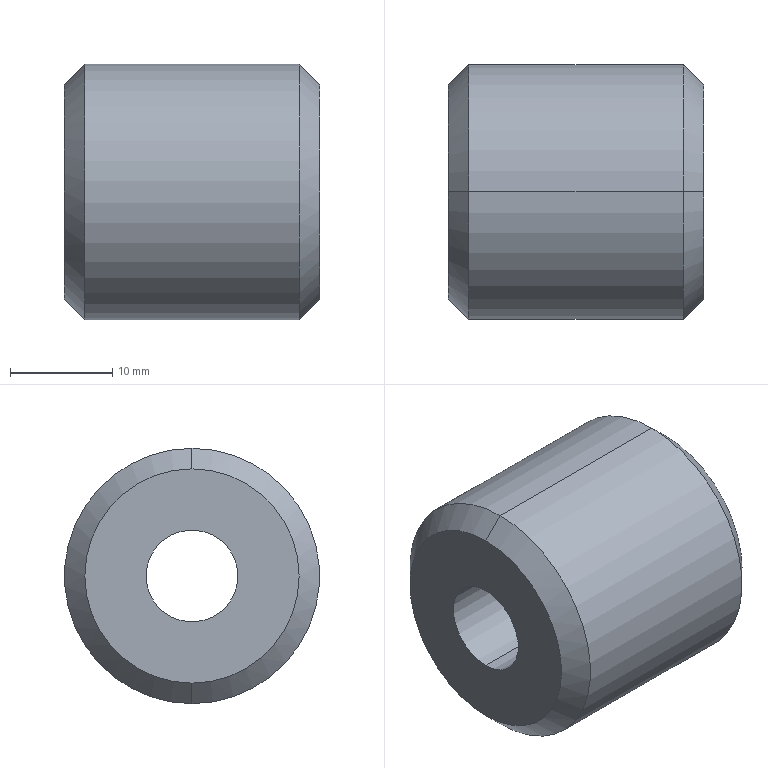Part | STEP file | LM-05-1235_default | 1 solid | 13 faces | box 25 x 25 x 25 mm | volume 9411 mm3 | cylinder 6 | cone 4 | plane 3 | commonest cylinder face diameters 9 x2 15 x2 25 x2
STEP:
#1=CARTESIAN_POINT('',(0.,0.,0.));
#2=DIRECTION('',(0.,0.,1.));
#3=DIRECTION('',(1.,0.,0.));
#4=AXIS2_PLACEMENT_3D('',#1,#2,#3);
#5=CARTESIAN_POINT('',(15.,0.,10.5));
#6=VERTEX_POINT('',#5);
#7=CARTESIAN_POINT('',(15.,0.,-10.5));
#8=VERTEX_POINT('',#7);
#9=CARTESIAN_POINT('',(15.,0.,0.));
#10=DIRECTION('',(-1.,0.,0.));
#11=DIRECTION('',(0.,0.,1.));
#12=AXIS2_PLACEMENT_3D('',#9,#10,#11);
#13=CIRCLE('',#12,10.5);
#14=CARTESIAN_POINT('',(13.,0.,0.));
#15=DIRECTION('',(-1.,0.,0.));
#16=DIRECTION('',(0.,0.,1.));
#17=AXIS2_PLACEMENT_3D('',#14,#15,#16);
#18=CONICAL_SURFACE('',#17,12.5,0.7854);
#19=CARTESIAN_POINT('',(0.,-2.));
#20=DIRECTION('',(1.,0.));
#21=VECTOR('',#20,1.);
#22=LINE('',#19,#21);
#23=(GEOMETRIC_REPRESENTATION_CONTEXT(2)PARAMETRIC_REPRESENTATION_CONTEXT()REPRESENTATION_CONTEXT('',''));
#24=DEFINITIONAL_REPRESENTATION('',(#22),#23);
#25=PCURVE('',#18,#24);
#26=CARTESIAN_POINT('',(15.,10.5,0.));
#27=DIRECTION('',(1.,0.,0.));
#28=DIRECTION('',(0.,0.,-1.));
#29=AXIS2_PLACEMENT_3D('',#26,#27,#28);
#30=PLANE('',#29);
#31=CARTESIAN_POINT('',(-10.5,-10.5));
#32=CARTESIAN_POINT('',(-10.5,7.687));
#33=CARTESIAN_POINT('',(5.25,-1.407));
#34=CARTESIAN_POINT('',(21.,-10.5));
#35=CARTESIAN_POINT('',(5.25,-19.593));
#36=CARTESIAN_POINT('',(-10.5,-28.687));
#37=CARTESIAN_POINT('',(-10.5,-10.5));
#38=(BOUNDED_CURVE()B_SPLINE_CURVE(2,(#31,#32,#33,#34,#35,#36,#37),.UNSPECIFIED.,.T.,.F.)B_SPLINE_CURVE_WITH_KNOTS((1,2,2,2,2,1),(-2.094,0.,2.094,4.189,6.283,8.378),.UNSPECIFIED.)CURVE()GEOMETRIC_REPRESENTATION_ITEM()RATIONAL_B_SPLINE_CURVE((1.,0.5,1.,0.5,1.,0.5,1.))REPRESENTATION_ITEM(''));
#39=(GEOMETRIC_REPRESENTATION_CONTEXT(2)PARAMETRIC_REPRESENTATION_CONTEXT()REPRESENTATION_CONTEXT('',''));
#40=DEFINITIONAL_REPRESENTATION('',(#38),#39);
#41=PCURVE('',#30,#40);
#42=SURFACE_CURVE('',#13,(#25,#41),.PCURVE_S1.);
#43=EDGE_CURVE('',#6,#8,#42,.T.);
#44=ORIENTED_EDGE('',*,*,#43,.T.);
#45=CARTESIAN_POINT('',(13.,0.,-12.5));
#46=VERTEX_POINT('',#45);
#47=CARTESIAN_POINT('',(13.,0.,-12.5));
#48=DIRECTION('',(-0.7071,0.,-0.7071));
#49=VECTOR('',#48,1.);
#50=LINE('',#47,#49);
#51=CARTESIAN_POINT('',(3.142,0.));
#52=DIRECTION('',(0.,1.));
#53=VECTOR('',#52,1.);
#54=LINE('',#51,#53);
#55=(GEOMETRIC_REPRESENTATION_CONTEXT(2)PARAMETRIC_REPRESENTATION_CONTEXT()REPRESENTATION_CONTEXT('',''));
#56=DEFINITIONAL_REPRESENTATION('',(#54),#55);
#57=PCURVE('',#18,#56);
#58=CARTESIAN_POINT('',(13.,0.,0.));
#59=DIRECTION('',(-1.,0.,0.));
#60=DIRECTION('',(0.,0.,1.));
#61=AXIS2_PLACEMENT_3D('',#58,#59,#60);
#62=CONICAL_SURFACE('',#61,12.5,0.7854);
#63=CARTESIAN_POINT('',(3.142,0.));
#64=DIRECTION('',(0.,1.));
#65=VECTOR('',#64,1.);
#66=LINE('',#63,#65);
#67=(GEOMETRIC_REPRESENTATION_CONTEXT(2)PARAMETRIC_REPRESENTATION_CONTEXT()REPRESENTATION_CONTEXT('',''));
#68=DEFINITIONAL_REPRESENTATION('',(#66),#67);
#69=PCURVE('',#62,#68);
#70=SURFACE_CURVE('',#50,(#57,#69),.PCURVE_S1.);
#71=EDGE_CURVE('',#8,#46,#70,.T.);
#72=ORIENTED_EDGE('',*,*,#71,.T.);
#73=CARTESIAN_POINT('',(13.,0.,12.5));
#74=VERTEX_POINT('',#73);
#75=CARTESIAN_POINT('',(13.,0.,0.));
#76=DIRECTION('',(-1.,0.,0.));
#77=DIRECTION('',(0.,0.,1.));
#78=AXIS2_PLACEMENT_3D('',#75,#76,#77);
#79=CIRCLE('',#78,12.5);
#80=CARTESIAN_POINT('',(0.,0.));
#81=DIRECTION('',(1.,0.));
#82=VECTOR('',#81,1.);
#83=LINE('',#80,#82);
#84=(GEOMETRIC_REPRESENTATION_CONTEXT(2)PARAMETRIC_REPRESENTATION_CONTEXT()REPRESENTATION_CONTEXT('',''));
#85=DEFINITIONAL_REPRESENTATION('',(#83),#84);
#86=PCURVE('',#18,#85);
#87=CARTESIAN_POINT('',(15.,0.,0.));
#88=DIRECTION('',(-1.,0.,0.));
#89=DIRECTION('',(0.,0.,1.));
#90=AXIS2_PLACEMENT_3D('',#87,#88,#89);
#91=CYLINDRICAL_SURFACE('',#90,12.5);
#92=CARTESIAN_POINT('',(0.,2.));
#93=DIRECTION('',(1.,0.));
#94=VECTOR('',#93,1.);
#95=LINE('',#92,#94);
#96=(GEOMETRIC_REPRESENTATION_CONTEXT(2)PARAMETRIC_REPRESENTATION_CONTEXT()REPRESENTATION_CONTEXT('',''));
#97=DEFINITIONAL_REPRESENTATION('',(#95),#96);
#98=PCURVE('',#91,#97);
#99=SURFACE_CURVE('',#79,(#86,#98),.PCURVE_S1.);
#100=EDGE_CURVE('',#74,#46,#99,.T.);
#101=ORIENTED_EDGE('',*,*,#100,.F.);
#102=CARTESIAN_POINT('',(13.,0.,12.5));
#103=DIRECTION('',(-0.7071,0.,0.7071));
#104=VECTOR('',#103,1.);
#105=LINE('',#102,#104);
#106=CARTESIAN_POINT('',(0.,0.));
#107=DIRECTION('',(0.,1.));
#108=VECTOR('',#107,1.);
#109=LINE('',#106,#108);
#110=(GEOMETRIC_REPRESENTATION_CONTEXT(2)PARAMETRIC_REPRESENTATION_CONTEXT()REPRESENTATION_CONTEXT('',''));
#111=DEFINITIONAL_REPRESENTATION('',(#109),#110);
#112=PCURVE('',#18,#111);
#113=CARTESIAN_POINT('',(6.283,0.));
#114=DIRECTION('',(0.,1.));
#115=VECTOR('',#114,1.);
#116=LINE('',#113,#115);
#117=(GEOMETRIC_REPRESENTATION_CONTEXT(2)PARAMETRIC_REPRESENTATION_CONTEXT()REPRESENTATION_CONTEXT('',''));
#118=DEFINITIONAL_REPRESENTATION('',(#116),#117);
#119=PCURVE('',#62,#118);
#120=SURFACE_CURVE('',#105,(#112,#119),.PCURVE_S1.);
#121=EDGE_CURVE('',#6,#74,#120,.T.);
#122=ORIENTED_EDGE('',*,*,#121,.F.);
#123=EDGE_LOOP('',(#44,#72,#101,#122));
#124=FACE_BOUND('',#123,.T.);
#125=ADVANCED_FACE('',(#124),#18,.T.);
#126=ORIENTED_EDGE('',*,*,#100,.T.);
#127=CARTESIAN_POINT('',(-8.,0.,-12.5));
#128=VERTEX_POINT('',#127);
#129=CARTESIAN_POINT('',(15.,0.,-12.5));
#130=DIRECTION('',(-1.,0.,0.));
#131=VECTOR('',#130,1.);
#132=LINE('',#129,#131);
#133=CARTESIAN_POINT('',(3.142,0.));
#134=DIRECTION('',(0.,1.));
#135=VECTOR('',#134,1.);
#136=LINE('',#133,#135);
#137=(GEOMETRIC_REPRESENTATION_CONTEXT(2)PARAMETRIC_REPRESENTATION_CONTEXT()REPRESENTATION_CONTEXT('',''));
#138=DEFINITIONAL_REPRESENTATION('',(#136),#137);
#139=PCURVE('',#91,#138);
#140=CARTESIAN_POINT('',(15.,0.,0.));
#141=DIRECTION('',(-1.,0.,0.));
#142=DIRECTION('',(0.,0.,1.));
#143=AXIS2_PLACEMENT_3D('',#140,#141,#142);
#144=CYLINDRICAL_SURFACE('',#143,12.5);
#145=CARTESIAN_POINT('',(3.142,0.));
#146=DIRECTION('',(0.,1.));
#147=VECTOR('',#146,1.);
#148=LINE('',#145,#147);
#149=(GEOMETRIC_REPRESENTATION_CONTEXT(2)PARAMETRIC_REPRESENTATION_CONTEXT()REPRESENTATION_CONTEXT('',''));
#150=DEFINITIONAL_REPRESENTATION('',(#148),#149);
#151=PCURVE('',#144,#150);
#152=SURFACE_CURVE('',#132,(#139,#151),.PCURVE_S1.);
#153=EDGE_CURVE('',#46,#128,#152,.T.);
#154=ORIENTED_EDGE('',*,*,#153,.T.);
#155=CARTESIAN_POINT('',(-8.,0.,12.5));
#156=VERTEX_POINT('',#155);
#157=CARTESIAN_POINT('',(-8.,0.,0.));
#158=DIRECTION('',(-1.,0.,0.));
#159=DIRECTION('',(0.,0.,1.));
#160=AXIS2_PLACEMENT_3D('',#157,#158,#159);
#161=CIRCLE('',#160,12.5);
#162=CARTESIAN_POINT('',(0.,23.));
#163=DIRECTION('',(1.,0.));
#164=VECTOR('',#163,1.);
#165=LINE('',#162,#164);
#166=(GEOMETRIC_REPRESENTATION_CONTEXT(2)PARAMETRIC_REPRESENTATION_CONTEXT()REPRESENTATION_CONTEXT('',''));
#167=DEFINITIONAL_REPRESENTATION('',(#165),#166);
#168=PCURVE('',#91,#167);
#169=CARTESIAN_POINT('',(-10.,0.,0.));
#170=DIRECTION('',(1.,0.,0.));
#171=DIRECTION('',(0.,0.,-1.));
#172=AXIS2_PLACEMENT_3D('',#169,#170,#171);
#173=CONICAL_SURFACE('',#172,10.5,0.7854);
#174=CARTESIAN_POINT('',(3.142,2.));
#175=DIRECTION('',(-1.,0.));
#176=VECTOR('',#175,1.);
#177=LINE('',#174,#176);
#178=(GEOMETRIC_REPRESENTATION_CONTEXT(2)PARAMETRIC_REPRESENTATION_CONTEXT()REPRESENTATION_CONTEXT('',''));
#179=DEFINITIONAL_REPRESENTATION('',(#177),#178);
#180=PCURVE('',#173,#179);
#181=SURFACE_CURVE('',#161,(#168,#180),.PCURVE_S1.);
#182=EDGE_CURVE('',#156,#128,#181,.T.);
#183=ORIENTED_EDGE('',*,*,#182,.F.);
#184=CARTESIAN_POINT('',(15.,0.,12.5));
#185=DIRECTION('',(-1.,0.,0.));
#186=VECTOR('',#185,1.);
#187=LINE('',#184,#186);
#188=CARTESIAN_POINT('',(0.,0.));
#189=DIRECTION('',(0.,1.));
#190=VECTOR('',#189,1.);
#191=LINE('',#188,#190);
#192=(GEOMETRIC_REPRESENTATION_CONTEXT(2)PARAMETRIC_REPRESENTATION_CONTEXT()REPRESENTATION_CONTEXT('',''));
#193=DEFINITIONAL_REPRESENTATION('',(#191),#192);
#194=PCURVE('',#91,#193);
#195=CARTESIAN_POINT('',(6.283,0.));
#196=DIRECTION('',(0.,1.));
#197=VECTOR('',#196,1.);
#198=LINE('',#195,#197);
#199=(GEOMETRIC_REPRESENTATION_CONTEXT(2)PARAMETRIC_REPRESENTATION_CONTEXT()REPRESENTATION_CONTEXT('',''));
#200=DEFINITIONAL_REPRESENTATION('',(#198),#199);
#201=PCURVE('',#144,#200);
#202=SURFACE_CURVE('',#187,(#194,#201),.PCURVE_S1.);
#203=EDGE_CURVE('',#74,#156,#202,.T.);
#204=ORIENTED_EDGE('',*,*,#203,.F.);
#205=EDGE_LOOP('',(#126,#154,#183,#204));
#206=FACE_BOUND('',#205,.T.);
#207=ADVANCED_FACE('',(#206),#91,.T.);
#208=CARTESIAN_POINT('',(-10.,0.,10.5));
#209=VERTEX_POINT('',#208);
#210=CARTESIAN_POINT('',(-10.,0.,-10.5));
#211=VERTEX_POINT('',#210);
#212=CARTESIAN_POINT('',(-10.,0.,0.));
#213=DIRECTION('',(-1.,0.,0.));
#214=DIRECTION('',(0.,0.,1.));
#215=AXIS2_PLACEMENT_3D('',#212,#213,#214);
#216=CIRCLE('',#215,10.5);
#217=CARTESIAN_POINT('',(3.142,0.));
#218=DIRECTION('',(-1.,0.));
#219=VECTOR('',#218,1.);
#220=LINE('',#217,#219);
#221=(GEOMETRIC_REPRESENTATION_CONTEXT(2)PARAMETRIC_REPRESENTATION_CONTEXT()REPRESENTATION_CONTEXT('',''));
#222=DEFINITIONAL_REPRESENTATION('',(#220),#221);
#223=PCURVE('',#173,#222);
#224=CARTESIAN_POINT('',(-10.,4.5,0.));
#225=DIRECTION('',(-1.,0.,0.));
#226=DIRECTION('',(0.,0.,1.));
#227=AXIS2_PLACEMENT_3D('',#224,#225,#226);
#228=PLANE('',#227);
#229=CARTESIAN_POINT('',(0.,-4.5));
#230=DIRECTION('',(1.,0.));
#231=AXIS2_PLACEMENT_2D('',#229,#230);
#232=CIRCLE('',#231,10.5);
#233=(GEOMETRIC_REPRESENTATION_CONTEXT(2)PARAMETRIC_REPRESENTATION_CONTEXT()REPRESENTATION_CONTEXT('',''));
#234=DEFINITIONAL_REPRESENTATION('',(#232),#233);
#235=PCURVE('',#228,#234);
#236=SURFACE_CURVE('',#216,(#223,#235),.PCURVE_S1.);
#237=EDGE_CURVE('',#209,#211,#236,.T.);
#238=ORIENTED_EDGE('',*,*,#237,.F.);
#239=CARTESIAN_POINT('',(-10.,0.,10.5));
#240=DIRECTION('',(0.7071,0.,0.7071));
#241=VECTOR('',#240,1.);
#242=LINE('',#239,#241);
#243=CARTESIAN_POINT('',(3.142,0.));
#244=DIRECTION('',(0.,1.));
#245=VECTOR('',#244,1.);
#246=LINE('',#243,#245);
#247=(GEOMETRIC_REPRESENTATION_CONTEXT(2)PARAMETRIC_REPRESENTATION_CONTEXT()REPRESENTATION_CONTEXT('',''));
#248=DEFINITIONAL_REPRESENTATION('',(#246),#247);
#249=PCURVE('',#173,#248);
#250=CARTESIAN_POINT('',(-10.,0.,0.));
#251=DIRECTION('',(1.,0.,0.));
#252=DIRECTION('',(0.,0.,-1.));
#253=AXIS2_PLACEMENT_3D('',#250,#251,#252);
#254=CONICAL_SURFACE('',#253,10.5,0.7854);
#255=CARTESIAN_POINT('',(3.142,0.));
#256=DIRECTION('',(0.,1.));
#257=VECTOR('',#256,1.);
#258=LINE('',#255,#257);
#259=(GEOMETRIC_REPRESENTATION_CONTEXT(2)PARAMETRIC_REPRESENTATION_CONTEXT()REPRESENTATION_CONTEXT('',''));
#260=DEFINITIONAL_REPRESENTATION('',(#258),#259);
#261=PCURVE('',#254,#260);
#262=SURFACE_CURVE('',#242,(#249,#261),.PCURVE_S1.);
#263=EDGE_CURVE('',#209,#156,#262,.T.);
#264=ORIENTED_EDGE('',*,*,#263,.T.);
#265=ORIENTED_EDGE('',*,*,#182,.T.);
#266=CARTESIAN_POINT('',(-10.,0.,-10.5));
#267=DIRECTION('',(0.7071,0.,-0.7071));
#268=VECTOR('',#267,1.);
#269=LINE('',#266,#268);
#270=CARTESIAN_POINT('',(0.,0.));
#271=DIRECTION('',(0.,1.));
#272=VECTOR('',#271,1.);
#273=LINE('',#270,#272);
#274=(GEOMETRIC_REPRESENTATION_CONTEXT(2)PARAMETRIC_REPRESENTATION_CONTEXT()REPRESENTATION_CONTEXT('',''));
#275=DEFINITIONAL_REPRESENTATION('',(#273),#274);
#276=PCURVE('',#173,#275);
#277=CARTESIAN_POINT('',(6.283,0.));
#278=DIRECTION('',(0.,1.));
#279=VECTOR('',#278,1.);
#280=LINE('',#277,#279);
#281=(GEOMETRIC_REPRESENTATION_CONTEXT(2)PARAMETRIC_REPRESENTATION_CONTEXT()REPRESENTATION_CONTEXT('',''));
#282=DEFINITIONAL_REPRESENTATION('',(#280),#281);
#283=PCURVE('',#254,#282);
#284=SURFACE_CURVE('',#269,(#276,#283),.PCURVE_S1.);
#285=EDGE_CURVE('',#211,#128,#284,.T.);
#286=ORIENTED_EDGE('',*,*,#285,.F.);
#287=EDGE_LOOP('',(#238,#264,#265,#286));
#288=FACE_BOUND('',#287,.T.);
#289=ADVANCED_FACE('',(#288),#173,.T.);
#290=CARTESIAN_POINT('',(6.4,0.,4.5));
#291=VERTEX_POINT('',#290);
#292=CARTESIAN_POINT('',(-10.,0.,4.5));
#293=VERTEX_POINT('',#292);
#294=CARTESIAN_POINT('',(15.,0.,4.5));
#295=DIRECTION('',(-1.,0.,0.));
#296=VECTOR('',#295,1.);
#297=LINE('',#294,#296);
#298=CARTESIAN_POINT('',(15.,0.,0.));
#299=DIRECTION('',(-1.,0.,0.));
#300=DIRECTION('',(0.,0.,1.));
#301=AXIS2_PLACEMENT_3D('',#298,#299,#300);
#302=CYLINDRICAL_SURFACE('',#301,4.5);
#303=CARTESIAN_POINT('',(6.283,0.));
#304=DIRECTION('',(0.,1.));
#305=VECTOR('',#304,1.);
#306=LINE('',#303,#305);
#307=(GEOMETRIC_REPRESENTATION_CONTEXT(2)PARAMETRIC_REPRESENTATION_CONTEXT()REPRESENTATION_CONTEXT('',''));
#308=DEFINITIONAL_REPRESENTATION('',(#306),#307);
#309=PCURVE('',#302,#308);
#310=CARTESIAN_POINT('',(15.,0.,0.));
#311=DIRECTION('',(-1.,0.,0.));
#312=DIRECTION('',(0.,0.,1.));
#313=AXIS2_PLACEMENT_3D('',#310,#311,#312);
#314=CYLINDRICAL_SURFACE('',#313,4.5);
#315=CARTESIAN_POINT('',(0.,0.));
#316=DIRECTION('',(0.,1.));
#317=VECTOR('',#316,1.);
#318=LINE('',#315,#317);
#319=(GEOMETRIC_REPRESENTATION_CONTEXT(2)PARAMETRIC_REPRESENTATION_CONTEXT()REPRESENTATION_CONTEXT('',''));
#320=DEFINITIONAL_REPRESENTATION('',(#318),#319);
#321=PCURVE('',#314,#320);
#322=SURFACE_CURVE('',#297,(#309,#321),.PCURVE_S1.);
#323=EDGE_CURVE('',#291,#293,#322,.T.);
#324=ORIENTED_EDGE('',*,*,#323,.T.);
#325=CARTESIAN_POINT('',(-10.,0.,-4.5));
#326=VERTEX_POINT('',#325);
#327=CARTESIAN_POINT('',(-10.,0.,0.));
#328=DIRECTION('',(-1.,0.,0.));
#329=DIRECTION('',(0.,0.,1.));
#330=AXIS2_PLACEMENT_3D('',#327,#328,#329);
#331=CIRCLE('',#330,4.5);
#332=CARTESIAN_POINT('',(0.,25.));
#333=DIRECTION('',(1.,0.));
#334=VECTOR('',#333,1.);
#335=LINE('',#332,#334);
#336=(GEOMETRIC_REPRESENTATION_CONTEXT(2)PARAMETRIC_REPRESENTATION_CONTEXT()REPRESENTATION_CONTEXT('',''));
#337=DEFINITIONAL_REPRESENTATION('',(#335),#336);
#338=PCURVE('',#302,#337);
#339=CARTESIAN_POINT('',(0.,-4.5));
#340=DIRECTION('',(1.,0.));
#341=AXIS2_PLACEMENT_2D('',#339,#340);
#342=CIRCLE('',#341,4.5);
#343=(GEOMETRIC_REPRESENTATION_CONTEXT(2)PARAMETRIC_REPRESENTATION_CONTEXT()REPRESENTATION_CONTEXT('',''));
#344=DEFINITIONAL_REPRESENTATION('',(#342),#343);
#345=PCURVE('',#228,#344);
#346=SURFACE_CURVE('',#331,(#338,#345),.PCURVE_S1.);
#347=EDGE_CURVE('',#326,#293,#346,.T.);
#348=ORIENTED_EDGE('',*,*,#347,.F.);
#349=CARTESIAN_POINT('',(6.4,0.,-4.5));
#350=VERTEX_POINT('',#349);
#351=CARTESIAN_POINT('',(15.,0.,-4.5));
#352=DIRECTION('',(-1.,0.,0.));
#353=VECTOR('',#352,1.);
#354=LINE('',#351,#353);
#355=CARTESIAN_POINT('',(3.142,0.));
#356=DIRECTION('',(0.,1.));
#357=VECTOR('',#356,1.);
#358=LINE('',#355,#357);
#359=(GEOMETRIC_REPRESENTATION_CONTEXT(2)PARAMETRIC_REPRESENTATION_CONTEXT()REPRESENTATION_CONTEXT('',''));
#360=DEFINITIONAL_REPRESENTATION('',(#358),#359);
#361=PCURVE('',#302,#360);
#362=CARTESIAN_POINT('',(3.142,0.));
#363=DIRECTION('',(0.,1.));
#364=VECTOR('',#363,1.);
#365=LINE('',#362,#364);
#366=(GEOMETRIC_REPRESENTATION_CONTEXT(2)PARAMETRIC_REPRESENTATION_CONTEXT()REPRESENTATION_CONTEXT('',''));
#367=DEFINITIONAL_REPRESENTATION('',(#365),#366);
#368=PCURVE('',#314,#367);
#369=SURFACE_CURVE('',#354,(#361,#368),.PCURVE_S1.);
#370=EDGE_CURVE('',#350,#326,#369,.T.);
#371=ORIENTED_EDGE('',*,*,#370,.F.);
#372=CARTESIAN_POINT('',(6.4,0.,0.));
#373=DIRECTION('',(-1.,0.,0.));
#374=DIRECTION('',(0.,0.,1.));
#375=AXIS2_PLACEMENT_3D('',#372,#373,#374);
#376=CIRCLE('',#375,4.5);
#377=CARTESIAN_POINT('',(0.,8.6));
#378=DIRECTION('',(1.,0.));
#379=VECTOR('',#378,1.);
#380=LINE('',#377,#379);
#381=(GEOMETRIC_REPRESENTATION_CONTEXT(2)PARAMETRIC_REPRESENTATION_CONTEXT()REPRESENTATION_CONTEXT('',''));
#382=DEFINITIONAL_REPRESENTATION('',(#380),#381);
#383=PCURVE('',#302,#382);
#384=CARTESIAN_POINT('',(6.4,7.5,0.));
#385=DIRECTION('',(1.,0.,0.));
#386=DIRECTION('',(0.,0.,-1.));
#387=AXIS2_PLACEMENT_3D('',#384,#385,#386);
#388=PLANE('',#387);
#389=CARTESIAN_POINT('',(-4.5,-7.5));
#390=CARTESIAN_POINT('',(-4.5,0.2942));
#391=CARTESIAN_POINT('',(2.25,-3.603));
#392=CARTESIAN_POINT('',(9.,-7.5));
#393=CARTESIAN_POINT('',(2.25,-11.397));
#394=CARTESIAN_POINT('',(-4.5,-15.294));
#395=CARTESIAN_POINT('',(-4.5,-7.5));
#396=(BOUNDED_CURVE()B_SPLINE_CURVE(2,(#389,#390,#391,#392,#393,#394,#395),.UNSPECIFIED.,.T.,.F.)B_SPLINE_CURVE_WITH_KNOTS((1,2,2,2,2,1),(-2.094,0.,2.094,4.189,6.283,8.378),.UNSPECIFIED.)CURVE()GEOMETRIC_REPRESENTATION_ITEM()RATIONAL_B_SPLINE_CURVE((1.,0.5,1.,0.5,1.,0.5,1.))REPRESENTATION_ITEM(''));
#397=(GEOMETRIC_REPRESENTATION_CONTEXT(2)PARAMETRIC_REPRESENTATION_CONTEXT()REPRESENTATION_CONTEXT('',''));
#398=DEFINITIONAL_REPRESENTATION('',(#396),#397);
#399=PCURVE('',#388,#398);
#400=SURFACE_CURVE('',#376,(#383,#399),.PCURVE_S1.);
#401=EDGE_CURVE('',#350,#291,#400,.T.);
#402=ORIENTED_EDGE('',*,*,#401,.T.);
#403=EDGE_LOOP('',(#324,#348,#371,#402));
#404=FACE_BOUND('',#403,.F.);
#405=ADVANCED_FACE('',(#404),#302,.F.);
#406=CARTESIAN_POINT('',(15.,0.,7.5));
#407=VERTEX_POINT('',#406);
#408=CARTESIAN_POINT('',(6.4,0.,7.5));
#409=VERTEX_POINT('',#408);
#410=CARTESIAN_POINT('',(15.,0.,7.5));
#411=DIRECTION('',(-1.,0.,0.));
#412=VECTOR('',#411,1.);
#413=LINE('',#410,#412);
#414=CARTESIAN_POINT('',(15.,0.,0.));
#415=DIRECTION('',(-1.,0.,0.));
#416=DIRECTION('',(0.,0.,1.));
#417=AXIS2_PLACEMENT_3D('',#414,#415,#416);
#418=CYLINDRICAL_SURFACE('',#417,7.5);
#419=CARTESIAN_POINT('',(6.283,0.));
#420=DIRECTION('',(0.,1.));
#421=VECTOR('',#420,1.);
#422=LINE('',#419,#421);
#423=(GEOMETRIC_REPRESENTATION_CONTEXT(2)PARAMETRIC_REPRESENTATION_CONTEXT()REPRESENTATION_CONTEXT('',''));
#424=DEFINITIONAL_REPRESENTATION('',(#422),#423);
#425=PCURVE('',#418,#424);
#426=CARTESIAN_POINT('',(15.,0.,0.));
#427=DIRECTION('',(-1.,0.,0.));
#428=DIRECTION('',(0.,0.,1.));
#429=AXIS2_PLACEMENT_3D('',#426,#427,#428);
#430=CYLINDRICAL_SURFACE('',#429,7.5);
#431=CARTESIAN_POINT('',(0.,0.));
#432=DIRECTION('',(0.,1.));
#433=VECTOR('',#432,1.);
#434=LINE('',#431,#433);
#435=(GEOMETRIC_REPRESENTATION_CONTEXT(2)PARAMETRIC_REPRESENTATION_CONTEXT()REPRESENTATION_CONTEXT('',''));
#436=DEFINITIONAL_REPRESENTATION('',(#434),#435);
#437=PCURVE('',#430,#436);
#438=SURFACE_CURVE('',#413,(#425,#437),.PCURVE_S1.);
#439=EDGE_CURVE('',#407,#409,#438,.T.);
#440=ORIENTED_EDGE('',*,*,#439,.T.);
#441=CARTESIAN_POINT('',(6.4,0.,-7.5));
#442=VERTEX_POINT('',#441);
#443=CARTESIAN_POINT('',(6.4,0.,0.));
#444=DIRECTION('',(-1.,0.,0.));
#445=DIRECTION('',(0.,0.,1.));
#446=AXIS2_PLACEMENT_3D('',#443,#444,#445);
#447=CIRCLE('',#446,7.5);
#448=CARTESIAN_POINT('',(0.,8.6));
#449=DIRECTION('',(1.,0.));
#450=VECTOR('',#449,1.);
#451=LINE('',#448,#450);
#452=(GEOMETRIC_REPRESENTATION_CONTEXT(2)PARAMETRIC_REPRESENTATION_CONTEXT()REPRESENTATION_CONTEXT('',''));
#453=DEFINITIONAL_REPRESENTATION('',(#451),#452);
#454=PCURVE('',#418,#453);
#455=CARTESIAN_POINT('',(-7.5,-7.5));
#456=CARTESIAN_POINT('',(-7.5,5.49));
#457=CARTESIAN_POINT('',(3.75,-1.005));
#458=CARTESIAN_POINT('',(15.,-7.5));
#459=CARTESIAN_POINT('',(3.75,-13.995));
#460=CARTESIAN_POINT('',(-7.5,-20.49));
#461=CARTESIAN_POINT('',(-7.5,-7.5));
#462=(BOUNDED_CURVE()B_SPLINE_CURVE(2,(#455,#456,#457,#458,#459,#460,#461),.UNSPECIFIED.,.T.,.F.)B_SPLINE_CURVE_WITH_KNOTS((1,2,2,2,2,1),(-2.094,0.,2.094,4.189,6.283,8.378),.UNSPECIFIED.)CURVE()GEOMETRIC_REPRESENTATION_ITEM()RATIONAL_B_SPLINE_CURVE((1.,0.5,1.,0.5,1.,0.5,1.))REPRESENTATION_ITEM(''));
#463=(GEOMETRIC_REPRESENTATION_CONTEXT(2)PARAMETRIC_REPRESENTATION_CONTEXT()REPRESENTATION_CONTEXT('',''));
#464=DEFINITIONAL_REPRESENTATION('',(#462),#463);
#465=PCURVE('',#388,#464);
#466=SURFACE_CURVE('',#447,(#454,#465),.PCURVE_S1.);
#467=EDGE_CURVE('',#442,#409,#466,.T.);
#468=ORIENTED_EDGE('',*,*,#467,.F.);
#469=CARTESIAN_POINT('',(15.,0.,-7.5));
#470=VERTEX_POINT('',#469);
#471=CARTESIAN_POINT('',(15.,0.,-7.5));
#472=DIRECTION('',(-1.,0.,0.));
#473=VECTOR('',#472,1.);
#474=LINE('',#471,#473);
#475=CARTESIAN_POINT('',(3.142,0.));
#476=DIRECTION('',(0.,1.));
#477=VECTOR('',#476,1.);
#478=LINE('',#475,#477);
#479=(GEOMETRIC_REPRESENTATION_CONTEXT(2)PARAMETRIC_REPRESENTATION_CONTEXT()REPRESENTATION_CONTEXT('',''));
#480=DEFINITIONAL_REPRESENTATION('',(#478),#479);
#481=PCURVE('',#418,#480);
#482=CARTESIAN_POINT('',(3.142,0.));
#483=DIRECTION('',(0.,1.));
#484=VECTOR('',#483,1.);
#485=LINE('',#482,#484);
#486=(GEOMETRIC_REPRESENTATION_CONTEXT(2)PARAMETRIC_REPRESENTATION_CONTEXT()REPRESENTATION_CONTEXT('',''));
#487=DEFINITIONAL_REPRESENTATION('',(#485),#486);
#488=PCURVE('',#430,#487);
#489=SURFACE_CURVE('',#474,(#481,#488),.PCURVE_S1.);
#490=EDGE_CURVE('',#470,#442,#489,.T.);
#491=ORIENTED_EDGE('',*,*,#490,.F.);
#492=CARTESIAN_POINT('',(15.,0.,0.));
#493=DIRECTION('',(-1.,0.,0.));
#494=DIRECTION('',(0.,0.,1.));
#495=AXIS2_PLACEMENT_3D('',#492,#493,#494);
#496=CIRCLE('',#495,7.5);
#497=CARTESIAN_POINT('',(0.,0.));
#498=DIRECTION('',(1.,0.));
#499=VECTOR('',#498,1.);
#500=LINE('',#497,#499);
#501=(GEOMETRIC_REPRESENTATION_CONTEXT(2)PARAMETRIC_REPRESENTATION_CONTEXT()REPRESENTATION_CONTEXT('',''));
#502=DEFINITIONAL_REPRESENTATION('',(#500),#501);
#503=PCURVE('',#418,#502);
#504=CARTESIAN_POINT('',(-7.5,-10.5));
#505=CARTESIAN_POINT('',(-7.5,2.49));
#506=CARTESIAN_POINT('',(3.75,-4.005));
#507=CARTESIAN_POINT('',(15.,-10.5));
#508=CARTESIAN_POINT('',(3.75,-16.995));
#509=CARTESIAN_POINT('',(-7.5,-23.49));
#510=CARTESIAN_POINT('',(-7.5,-10.5));
#511=(BOUNDED_CURVE()B_SPLINE_CURVE(2,(#504,#505,#506,#507,#508,#509,#510),.UNSPECIFIED.,.T.,.F.)B_SPLINE_CURVE_WITH_KNOTS((1,2,2,2,2,1),(-2.094,0.,2.094,4.189,6.283,8.378),.UNSPECIFIED.)CURVE()GEOMETRIC_REPRESENTATION_ITEM()RATIONAL_B_SPLINE_CURVE((1.,0.5,1.,0.5,1.,0.5,1.))REPRESENTATION_ITEM(''));
#512=(GEOMETRIC_REPRESENTATION_CONTEXT(2)PARAMETRIC_REPRESENTATION_CONTEXT()REPRESENTATION_CONTEXT('',''));
#513=DEFINITIONAL_REPRESENTATION('',(#511),#512);
#514=PCURVE('',#30,#513);
#515=SURFACE_CURVE('',#496,(#503,#514),.PCURVE_S1.);
#516=EDGE_CURVE('',#470,#407,#515,.T.);
#517=ORIENTED_EDGE('',*,*,#516,.T.);
#518=EDGE_LOOP('',(#440,#468,#491,#517));
#519=FACE_BOUND('',#518,.F.);
#520=ADVANCED_FACE('',(#519),#418,.F.);
#521=CARTESIAN_POINT('',(15.,0.,0.));
#522=DIRECTION('',(-1.,0.,0.));
#523=DIRECTION('',(0.,0.,1.));
#524=AXIS2_PLACEMENT_3D('',#521,#522,#523);
#525=CIRCLE('',#524,7.5);
#526=CARTESIAN_POINT('',(-7.5,-10.5));
#527=CARTESIAN_POINT('',(-7.5,2.49));
#528=CARTESIAN_POINT('',(3.75,-4.005));
#529=CARTESIAN_POINT('',(15.,-10.5));
#530=CARTESIAN_POINT('',(3.75,-16.995));
#531=CARTESIAN_POINT('',(-7.5,-23.49));
#532=CARTESIAN_POINT('',(-7.5,-10.5));
#533=(BOUNDED_CURVE()B_SPLINE_CURVE(2,(#526,#527,#528,#529,#530,#531,#532),.UNSPECIFIED.,.T.,.F.)B_SPLINE_CURVE_WITH_KNOTS((1,2,2,2,2,1),(-2.094,0.,2.094,4.189,6.283,8.378),.UNSPECIFIED.)CURVE()GEOMETRIC_REPRESENTATION_ITEM()RATIONAL_B_SPLINE_CURVE((1.,0.5,1.,0.5,1.,0.5,1.))REPRESENTATION_ITEM(''));
#534=(GEOMETRIC_REPRESENTATION_CONTEXT(2)PARAMETRIC_REPRESENTATION_CONTEXT()REPRESENTATION_CONTEXT('',''));
#535=DEFINITIONAL_REPRESENTATION('',(#533),#534);
#536=PCURVE('',#30,#535);
#537=CARTESIAN_POINT('',(0.,0.));
#538=DIRECTION('',(1.,0.));
#539=VECTOR('',#538,1.);
#540=LINE('',#537,#539);
#541=(GEOMETRIC_REPRESENTATION_CONTEXT(2)PARAMETRIC_REPRESENTATION_CONTEXT()REPRESENTATION_CONTEXT('',''));
#542=DEFINITIONAL_REPRESENTATION('',(#540),#541);
#543=PCURVE('',#430,#542);
#544=SURFACE_CURVE('',#525,(#536,#543),.PCURVE_S1.);
#545=EDGE_CURVE('',#407,#470,#544,.T.);
#546=ORIENTED_EDGE('',*,*,#545,.T.);
#547=ORIENTED_EDGE('',*,*,#516,.T.);
#548=EDGE_LOOP('',(#546,#547));
#549=FACE_BOUND('',#548,.T.);
#550=ORIENTED_EDGE('',*,*,#43,.F.);
#551=CARTESIAN_POINT('',(15.,0.,0.));
#552=DIRECTION('',(-1.,0.,0.));
#553=DIRECTION('',(0.,0.,1.));
#554=AXIS2_PLACEMENT_3D('',#551,#552,#553);
#555=CIRCLE('',#554,10.5);
#556=CARTESIAN_POINT('',(-10.5,-10.5));
#557=CARTESIAN_POINT('',(-10.5,7.687));
#558=CARTESIAN_POINT('',(5.25,-1.407));
#559=CARTESIAN_POINT('',(21.,-10.5));
#560=CARTESIAN_POINT('',(5.25,-19.593));
#561=CARTESIAN_POINT('',(-10.5,-28.687));
#562=CARTESIAN_POINT('',(-10.5,-10.5));
#563=(BOUNDED_CURVE()B_SPLINE_CURVE(2,(#556,#557,#558,#559,#560,#561,#562),.UNSPECIFIED.,.T.,.F.)B_SPLINE_CURVE_WITH_KNOTS((1,2,2,2,2,1),(-2.094,0.,2.094,4.189,6.283,8.378),.UNSPECIFIED.)CURVE()GEOMETRIC_REPRESENTATION_ITEM()RATIONAL_B_SPLINE_CURVE((1.,0.5,1.,0.5,1.,0.5,1.))REPRESENTATION_ITEM(''));
#564=(GEOMETRIC_REPRESENTATION_CONTEXT(2)PARAMETRIC_REPRESENTATION_CONTEXT()REPRESENTATION_CONTEXT('',''));
#565=DEFINITIONAL_REPRESENTATION('',(#563),#564);
#566=PCURVE('',#30,#565);
#567=CARTESIAN_POINT('',(0.,-2.));
#568=DIRECTION('',(1.,0.));
#569=VECTOR('',#568,1.);
#570=LINE('',#567,#569);
#571=(GEOMETRIC_REPRESENTATION_CONTEXT(2)PARAMETRIC_REPRESENTATION_CONTEXT()REPRESENTATION_CONTEXT('',''));
#572=DEFINITIONAL_REPRESENTATION('',(#570),#571);
#573=PCURVE('',#62,#572);
#574=SURFACE_CURVE('',#555,(#566,#573),.PCURVE_S1.);
#575=EDGE_CURVE('',#8,#6,#574,.T.);
#576=ORIENTED_EDGE('',*,*,#575,.F.);
#577=EDGE_LOOP('',(#550,#576));
#578=FACE_BOUND('',#577,.T.);
#579=ADVANCED_FACE('',(#549,#578),#30,.T.);
#580=CARTESIAN_POINT('',(6.4,0.,0.));
#581=DIRECTION('',(-1.,0.,0.));
#582=DIRECTION('',(0.,0.,1.));
#583=AXIS2_PLACEMENT_3D('',#580,#581,#582);
#584=CIRCLE('',#583,7.5);
#585=CARTESIAN_POINT('',(0.,8.6));
#586=DIRECTION('',(1.,0.));
#587=VECTOR('',#586,1.);
#588=LINE('',#585,#587);
#589=(GEOMETRIC_REPRESENTATION_CONTEXT(2)PARAMETRIC_REPRESENTATION_CONTEXT()REPRESENTATION_CONTEXT('',''));
#590=DEFINITIONAL_REPRESENTATION('',(#588),#589);
#591=PCURVE('',#430,#590);
#592=CARTESIAN_POINT('',(-7.5,-7.5));
#593=CARTESIAN_POINT('',(-7.5,5.49));
#594=CARTESIAN_POINT('',(3.75,-1.005));
#595=CARTESIAN_POINT('',(15.,-7.5));
#596=CARTESIAN_POINT('',(3.75,-13.995));
#597=CARTESIAN_POINT('',(-7.5,-20.49));
#598=CARTESIAN_POINT('',(-7.5,-7.5));
#599=(BOUNDED_CURVE()B_SPLINE_CURVE(2,(#592,#593,#594,#595,#596,#597,#598),.UNSPECIFIED.,.T.,.F.)B_SPLINE_CURVE_WITH_KNOTS((1,2,2,2,2,1),(-2.094,0.,2.094,4.189,6.283,8.378),.UNSPECIFIED.)CURVE()GEOMETRIC_REPRESENTATION_ITEM()RATIONAL_B_SPLINE_CURVE((1.,0.5,1.,0.5,1.,0.5,1.))REPRESENTATION_ITEM(''));
#600=(GEOMETRIC_REPRESENTATION_CONTEXT(2)PARAMETRIC_REPRESENTATION_CONTEXT()REPRESENTATION_CONTEXT('',''));
#601=DEFINITIONAL_REPRESENTATION('',(#599),#600);
#602=PCURVE('',#388,#601);
#603=SURFACE_CURVE('',#584,(#591,#602),.PCURVE_S1.);
#604=EDGE_CURVE('',#409,#442,#603,.T.);
#605=ORIENTED_EDGE('',*,*,#604,.F.);
#606=ORIENTED_EDGE('',*,*,#439,.F.);
#607=ORIENTED_EDGE('',*,*,#545,.T.);
#608=ORIENTED_EDGE('',*,*,#490,.T.);
#609=EDGE_LOOP('',(#605,#606,#607,#608));
#610=FACE_BOUND('',#609,.F.);
#611=ADVANCED_FACE('',(#610),#430,.F.);
#612=CARTESIAN_POINT('',(6.4,0.,0.));
#613=DIRECTION('',(-1.,0.,0.));
#614=DIRECTION('',(0.,0.,1.));
#615=AXIS2_PLACEMENT_3D('',#612,#613,#614);
#616=CIRCLE('',#615,4.5);
#617=CARTESIAN_POINT('',(-4.5,-7.5));
#618=CARTESIAN_POINT('',(-4.5,0.2942));
#619=CARTESIAN_POINT('',(2.25,-3.603));
#620=CARTESIAN_POINT('',(9.,-7.5));
#621=CARTESIAN_POINT('',(2.25,-11.397));
#622=CARTESIAN_POINT('',(-4.5,-15.294));
#623=CARTESIAN_POINT('',(-4.5,-7.5));
#624=(BOUNDED_CURVE()B_SPLINE_CURVE(2,(#617,#618,#619,#620,#621,#622,#623),.UNSPECIFIED.,.T.,.F.)B_SPLINE_CURVE_WITH_KNOTS((1,2,2,2,2,1),(-2.094,0.,2.094,4.189,6.283,8.378),.UNSPECIFIED.)CURVE()GEOMETRIC_REPRESENTATION_ITEM()RATIONAL_B_SPLINE_CURVE((1.,0.5,1.,0.5,1.,0.5,1.))REPRESENTATION_ITEM(''));
#625=(GEOMETRIC_REPRESENTATION_CONTEXT(2)PARAMETRIC_REPRESENTATION_CONTEXT()REPRESENTATION_CONTEXT('',''));
#626=DEFINITIONAL_REPRESENTATION('',(#624),#625);
#627=PCURVE('',#388,#626);
#628=CARTESIAN_POINT('',(0.,8.6));
#629=DIRECTION('',(1.,0.));
#630=VECTOR('',#629,1.);
#631=LINE('',#628,#630);
#632=(GEOMETRIC_REPRESENTATION_CONTEXT(2)PARAMETRIC_REPRESENTATION_CONTEXT()REPRESENTATION_CONTEXT('',''));
#633=DEFINITIONAL_REPRESENTATION('',(#631),#632);
#634=PCURVE('',#314,#633);
#635=SURFACE_CURVE('',#616,(#627,#634),.PCURVE_S1.);
#636=EDGE_CURVE('',#291,#350,#635,.T.);
#637=ORIENTED_EDGE('',*,*,#636,.T.);
#638=ORIENTED_EDGE('',*,*,#401,.T.);
#639=EDGE_LOOP('',(#637,#638));
#640=FACE_BOUND('',#639,.T.);
#641=ORIENTED_EDGE('',*,*,#604,.F.);
#642=ORIENTED_EDGE('',*,*,#467,.F.);
#643=EDGE_LOOP('',(#641,#642));
#644=FACE_BOUND('',#643,.T.);
#645=ADVANCED_FACE('',(#640,#644),#388,.T.);
#646=CARTESIAN_POINT('',(-10.,0.,0.));
#647=DIRECTION('',(-1.,0.,0.));
#648=DIRECTION('',(0.,0.,1.));
#649=AXIS2_PLACEMENT_3D('',#646,#647,#648);
#650=CIRCLE('',#649,4.5);
#651=CARTESIAN_POINT('',(0.,25.));
#652=DIRECTION('',(1.,0.));
#653=VECTOR('',#652,1.);
#654=LINE('',#651,#653);
#655=(GEOMETRIC_REPRESENTATION_CONTEXT(2)PARAMETRIC_REPRESENTATION_CONTEXT()REPRESENTATION_CONTEXT('',''));
#656=DEFINITIONAL_REPRESENTATION('',(#654),#655);
#657=PCURVE('',#314,#656);
#658=CARTESIAN_POINT('',(0.,-4.5));
#659=DIRECTION('',(1.,0.));
#660=AXIS2_PLACEMENT_2D('',#658,#659);
#661=CIRCLE('',#660,4.5);
#662=(GEOMETRIC_REPRESENTATION_CONTEXT(2)PARAMETRIC_REPRESENTATION_CONTEXT()REPRESENTATION_CONTEXT('',''));
#663=DEFINITIONAL_REPRESENTATION('',(#661),#662);
#664=PCURVE('',#228,#663);
#665=SURFACE_CURVE('',#650,(#657,#664),.PCURVE_S1.);
#666=EDGE_CURVE('',#293,#326,#665,.T.);
#667=ORIENTED_EDGE('',*,*,#666,.F.);
#668=ORIENTED_EDGE('',*,*,#323,.F.);
#669=ORIENTED_EDGE('',*,*,#636,.T.);
#670=ORIENTED_EDGE('',*,*,#370,.T.);
#671=EDGE_LOOP('',(#667,#668,#669,#670));
#672=FACE_BOUND('',#671,.F.);
#673=ADVANCED_FACE('',(#672),#314,.F.);
#674=CARTESIAN_POINT('',(-10.,0.,0.));
#675=DIRECTION('',(-1.,0.,0.));
#676=DIRECTION('',(0.,0.,1.));
#677=AXIS2_PLACEMENT_3D('',#674,#675,#676);
#678=CIRCLE('',#677,10.5);
#679=CARTESIAN_POINT('',(0.,-4.5));
#680=DIRECTION('',(1.,0.));
#681=AXIS2_PLACEMENT_2D('',#679,#680);
#682=CIRCLE('',#681,10.5);
#683=(GEOMETRIC_REPRESENTATION_CONTEXT(2)PARAMETRIC_REPRESENTATION_CONTEXT()REPRESENTATION_CONTEXT('',''));
#684=DEFINITIONAL_REPRESENTATION('',(#682),#683);
#685=PCURVE('',#228,#684);
#686=CARTESIAN_POINT('',(9.425,0.));
#687=DIRECTION('',(-1.,0.));
#688=VECTOR('',#687,1.);
#689=LINE('',#686,#688);
#690=(GEOMETRIC_REPRESENTATION_CONTEXT(2)PARAMETRIC_REPRESENTATION_CONTEXT()REPRESENTATION_CONTEXT('',''));
#691=DEFINITIONAL_REPRESENTATION('',(#689),#690);
#692=PCURVE('',#254,#691);
#693=SURFACE_CURVE('',#678,(#685,#692),.PCURVE_S1.);
#694=EDGE_CURVE('',#211,#209,#693,.T.);
#695=ORIENTED_EDGE('',*,*,#694,.T.);
#696=ORIENTED_EDGE('',*,*,#237,.T.);
#697=EDGE_LOOP('',(#695,#696));
#698=FACE_BOUND('',#697,.T.);
#699=ORIENTED_EDGE('',*,*,#666,.F.);
#700=ORIENTED_EDGE('',*,*,#347,.F.);
#701=EDGE_LOOP('',(#699,#700));
#702=FACE_BOUND('',#701,.T.);
#703=ADVANCED_FACE('',(#698,#702),#228,.T.);
#704=ORIENTED_EDGE('',*,*,#263,.F.);
#705=ORIENTED_EDGE('',*,*,#694,.F.);
#706=ORIENTED_EDGE('',*,*,#285,.T.);
#707=CARTESIAN_POINT('',(-8.,0.,0.));
#708=DIRECTION('',(-1.,0.,0.));
#709=DIRECTION('',(0.,0.,1.));
#710=AXIS2_PLACEMENT_3D('',#707,#708,#709);
#711=CIRCLE('',#710,12.5);
#712=CARTESIAN_POINT('',(9.425,2.));
#713=DIRECTION('',(-1.,0.));
#714=VECTOR('',#713,1.);
#715=LINE('',#712,#714);
#716=(GEOMETRIC_REPRESENTATION_CONTEXT(2)PARAMETRIC_REPRESENTATION_CONTEXT()REPRESENTATION_CONTEXT('',''));
#717=DEFINITIONAL_REPRESENTATION('',(#715),#716);
#718=PCURVE('',#254,#717);
#719=CARTESIAN_POINT('',(0.,23.));
#720=DIRECTION('',(1.,0.));
#721=VECTOR('',#720,1.);
#722=LINE('',#719,#721);
#723=(GEOMETRIC_REPRESENTATION_CONTEXT(2)PARAMETRIC_REPRESENTATION_CONTEXT()REPRESENTATION_CONTEXT('',''));
#724=DEFINITIONAL_REPRESENTATION('',(#722),#723);
#725=PCURVE('',#144,#724);
#726=SURFACE_CURVE('',#711,(#718,#725),.PCURVE_S1.);
#727=EDGE_CURVE('',#128,#156,#726,.T.);
#728=ORIENTED_EDGE('',*,*,#727,.T.);
#729=EDGE_LOOP('',(#704,#705,#706,#728));
#730=FACE_BOUND('',#729,.T.);
#731=ADVANCED_FACE('',(#730),#254,.T.);
#732=ORIENTED_EDGE('',*,*,#153,.F.);
#733=CARTESIAN_POINT('',(13.,0.,0.));
#734=DIRECTION('',(-1.,0.,0.));
#735=DIRECTION('',(0.,0.,1.));
#736=AXIS2_PLACEMENT_3D('',#733,#734,#735);
#737=CIRCLE('',#736,12.5);
#738=CARTESIAN_POINT('',(0.,2.));
#739=DIRECTION('',(1.,0.));
#740=VECTOR('',#739,1.);
#741=LINE('',#738,#740);
#742=(GEOMETRIC_REPRESENTATION_CONTEXT(2)PARAMETRIC_REPRESENTATION_CONTEXT()REPRESENTATION_CONTEXT('',''));
#743=DEFINITIONAL_REPRESENTATION('',(#741),#742);
#744=PCURVE('',#144,#743);
#745=CARTESIAN_POINT('',(0.,0.));
#746=DIRECTION('',(1.,0.));
#747=VECTOR('',#746,1.);
#748=LINE('',#745,#747);
#749=(GEOMETRIC_REPRESENTATION_CONTEXT(2)PARAMETRIC_REPRESENTATION_CONTEXT()REPRESENTATION_CONTEXT('',''));
#750=DEFINITIONAL_REPRESENTATION('',(#748),#749);
#751=PCURVE('',#62,#750);
#752=SURFACE_CURVE('',#737,(#744,#751),.PCURVE_S1.);
#753=EDGE_CURVE('',#46,#74,#752,.T.);
#754=ORIENTED_EDGE('',*,*,#753,.T.);
#755=ORIENTED_EDGE('',*,*,#203,.T.);
#756=ORIENTED_EDGE('',*,*,#727,.F.);
#757=EDGE_LOOP('',(#732,#754,#755,#756));
#758=FACE_BOUND('',#757,.T.);
#759=ADVANCED_FACE('',(#758),#144,.T.);
#760=ORIENTED_EDGE('',*,*,#71,.F.);
#761=ORIENTED_EDGE('',*,*,#575,.T.);
#762=ORIENTED_EDGE('',*,*,#121,.T.);
#763=ORIENTED_EDGE('',*,*,#753,.F.);
#764=EDGE_LOOP('',(#760,#761,#762,#763));
#765=FACE_BOUND('',#764,.T.);
#766=ADVANCED_FACE('',(#765),#62,.T.);
#767=CLOSED_SHELL('',(#125,#207,#289,#405,#520,#579,#611,#645,#673,#703,#731,#759,#766));
#768=MANIFOLD_SOLID_BREP('',#767);
#769=(LENGTH_UNIT()NAMED_UNIT(*)SI_UNIT(.MILLI.,.METRE.));
#770=UNCERTAINTY_MEASURE_WITH_UNIT(LENGTH_MEASURE(0.0000001),#769,'','');
#771=(NAMED_UNIT(*)PLANE_ANGLE_UNIT()SI_UNIT($,.RADIAN.));
#772=(NAMED_UNIT(*)SI_UNIT($,.STERADIAN.)SOLID_ANGLE_UNIT());
#773=(GEOMETRIC_REPRESENTATION_CONTEXT(3)GLOBAL_UNCERTAINTY_ASSIGNED_CONTEXT((#770))GLOBAL_UNIT_ASSIGNED_CONTEXT((#769,#771,#772))REPRESENTATION_CONTEXT('',''));
#774=ADVANCED_BREP_SHAPE_REPRESENTATION('',(#4,#768),#773);